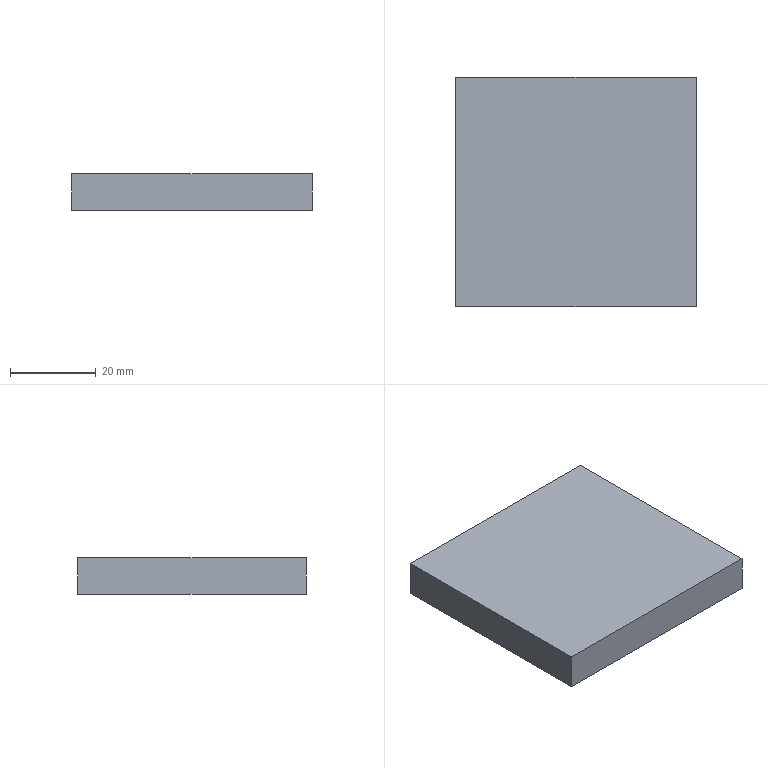Part | 2 solids | 162 faces | box 56 x 53.3 x 8.5 mm | volume 22053 mm3 | cylinder 123 | plane 39 | commonest cylinder face diameters 2 x20 5 x18 4 x17 43.3 x12 4.1 x10 3 x9